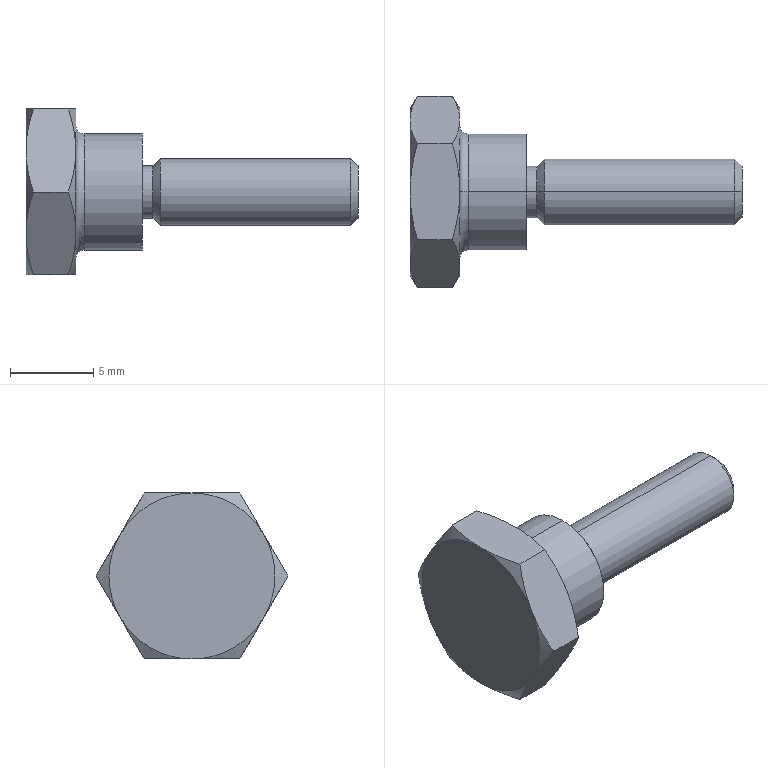Part | STEP file | 11-FJTM4_0_7_413part111 | 1 solid | 34 faces | box 20 x 11.547 x 10 mm | volume 570.86 mm3 | cone 16 | plane 10 | cylinder 6 | torus 2 | commonest cylinder face diameters 3.141 x2 4 x2 7 x2
STEP:
#1=CARTESIAN_POINT('',(3.,0.,-4.));
#2=VERTEX_POINT('',#1);
#3=CARTESIAN_POINT('',(3.,0.,4.));
#4=VERTEX_POINT('',#3);
#5=CARTESIAN_POINT('',(3.,0.,0.));
#6=DIRECTION('',(-1.,0.,0.));
#7=DIRECTION('',(0.,0.,1.));
#8=AXIS2_PLACEMENT_3D('',#5,#6,#7);
#9=CIRCLE('',#8,4.);
#10=EDGE_CURVE('',#2,#4,#9,.T.);
#11=ORIENTED_EDGE('',*,*,#10,.F.);
#12=CARTESIAN_POINT('',(3.5,0.,-3.5));
#13=VERTEX_POINT('',#12);
#14=CARTESIAN_POINT('',(3.5,0.,-4.));
#15=DIRECTION('',(0.,1.,0.));
#16=DIRECTION('',(0.,0.,1.));
#17=AXIS2_PLACEMENT_3D('',#14,#15,#16);
#18=CIRCLE('',#17,0.5);
#19=EDGE_CURVE('',#2,#13,#18,.T.);
#20=ORIENTED_EDGE('',*,*,#19,.T.);
#21=CARTESIAN_POINT('',(3.5,0.,3.5));
#22=VERTEX_POINT('',#21);
#23=CARTESIAN_POINT('',(3.5,0.,0.));
#24=DIRECTION('',(-1.,0.,0.));
#25=DIRECTION('',(0.,0.,1.));
#26=AXIS2_PLACEMENT_3D('',#23,#24,#25);
#27=CIRCLE('',#26,3.5);
#28=EDGE_CURVE('',#13,#22,#27,.T.);
#29=ORIENTED_EDGE('',*,*,#28,.T.);
#30=CARTESIAN_POINT('',(3.5,0.,4.));
#31=DIRECTION('',(0.,-1.,0.));
#32=DIRECTION('',(0.,0.,-1.));
#33=AXIS2_PLACEMENT_3D('',#30,#31,#32);
#34=CIRCLE('',#33,0.5);
#35=EDGE_CURVE('',#4,#22,#34,.T.);
#36=ORIENTED_EDGE('',*,*,#35,.F.);
#37=EDGE_LOOP('',(#11,#20,#29,#36));
#38=FACE_OUTER_BOUND('',#37,.T.);
#39=CARTESIAN_POINT('',(3.5,0.,0.));
#40=DIRECTION('',(-1.,0.,0.));
#41=DIRECTION('',(0.,0.,1.));
#42=AXIS2_PLACEMENT_3D('',#39,#40,#41);
#43=TOROIDAL_SURFACE('',#42,4.,0.5);
#44=ADVANCED_FACE('',(#38),#43,.F.);
#45=CARTESIAN_POINT('',(7.,0.,3.5));
#46=VERTEX_POINT('',#45);
#47=CARTESIAN_POINT('',(7.,0.,-3.5));
#48=VERTEX_POINT('',#47);
#49=CARTESIAN_POINT('',(7.,0.,0.));
#50=DIRECTION('',(-1.,0.,0.));
#51=DIRECTION('',(0.,0.,1.));
#52=AXIS2_PLACEMENT_3D('',#49,#50,#51);
#53=CIRCLE('',#52,3.5);
#54=EDGE_CURVE('',#46,#48,#53,.T.);
#55=ORIENTED_EDGE('',*,*,#54,.T.);
#56=CARTESIAN_POINT('',(20.,0.,-3.5));
#57=DIRECTION('',(-1.,0.,0.));
#58=VECTOR('',#57,1000.);
#59=LINE('',#56,#58);
#60=EDGE_CURVE('',#48,#13,#59,.T.);
#61=ORIENTED_EDGE('',*,*,#60,.T.);
#62=CARTESIAN_POINT('',(3.5,0.,0.));
#63=DIRECTION('',(-1.,0.,0.));
#64=DIRECTION('',(0.,0.,1.));
#65=AXIS2_PLACEMENT_3D('',#62,#63,#64);
#66=CIRCLE('',#65,3.5);
#67=EDGE_CURVE('',#22,#13,#66,.T.);
#68=ORIENTED_EDGE('',*,*,#67,.F.);
#69=CARTESIAN_POINT('',(20.,0.,3.5));
#70=DIRECTION('',(-1.,0.,0.));
#71=VECTOR('',#70,1000.);
#72=LINE('',#69,#71);
#73=EDGE_CURVE('',#46,#22,#72,.T.);
#74=ORIENTED_EDGE('',*,*,#73,.F.);
#75=EDGE_LOOP('',(#55,#61,#68,#74));
#76=FACE_OUTER_BOUND('',#75,.T.);
#77=CARTESIAN_POINT('',(20.,0.,0.));
#78=DIRECTION('',(-1.,0.,0.));
#79=DIRECTION('',(0.,0.,1.));
#80=AXIS2_PLACEMENT_3D('',#77,#78,#79);
#81=CYLINDRICAL_SURFACE('',#80,3.5);
#82=ADVANCED_FACE('',(#76),#81,.T.);
#83=CARTESIAN_POINT('',(7.65,0.,1.571));
#84=VERTEX_POINT('',#83);
#85=CARTESIAN_POINT('',(7.65,0.,-1.571));
#86=VERTEX_POINT('',#85);
#87=CARTESIAN_POINT('',(7.65,0.,0.));
#88=DIRECTION('',(-1.,0.,0.));
#89=DIRECTION('',(0.,0.,1.));
#90=AXIS2_PLACEMENT_3D('',#87,#88,#89);
#91=CIRCLE('',#90,1.571);
#92=EDGE_CURVE('',#84,#86,#91,.T.);
#93=ORIENTED_EDGE('',*,*,#92,.T.);
#94=CARTESIAN_POINT('',(7.,0.,-1.571));
#95=VERTEX_POINT('',#94);
#96=CARTESIAN_POINT('',(20.,0.,-1.571));
#97=DIRECTION('',(-1.,0.,0.));
#98=VECTOR('',#97,1000.);
#99=LINE('',#96,#98);
#100=EDGE_CURVE('',#86,#95,#99,.T.);
#101=ORIENTED_EDGE('',*,*,#100,.T.);
#102=CARTESIAN_POINT('',(7.,0.,1.571));
#103=VERTEX_POINT('',#102);
#104=CARTESIAN_POINT('',(7.,0.,0.));
#105=DIRECTION('',(-1.,0.,0.));
#106=DIRECTION('',(0.,0.,1.));
#107=AXIS2_PLACEMENT_3D('',#104,#105,#106);
#108=CIRCLE('',#107,1.571);
#109=EDGE_CURVE('',#103,#95,#108,.T.);
#110=ORIENTED_EDGE('',*,*,#109,.F.);
#111=CARTESIAN_POINT('',(20.,0.,1.571));
#112=DIRECTION('',(-1.,0.,0.));
#113=VECTOR('',#112,1000.);
#114=LINE('',#111,#113);
#115=EDGE_CURVE('',#84,#103,#114,.T.);
#116=ORIENTED_EDGE('',*,*,#115,.F.);
#117=EDGE_LOOP('',(#93,#101,#110,#116));
#118=FACE_OUTER_BOUND('',#117,.T.);
#119=CARTESIAN_POINT('',(20.,0.,0.));
#120=DIRECTION('',(-1.,0.,0.));
#121=DIRECTION('',(0.,0.,1.));
#122=AXIS2_PLACEMENT_3D('',#119,#120,#121);
#123=CYLINDRICAL_SURFACE('',#122,1.571);
#124=ADVANCED_FACE('',(#118),#123,.T.);
#125=ORIENTED_EDGE('',*,*,#92,.F.);
#126=CARTESIAN_POINT('',(8.079,0.,2.));
#127=VERTEX_POINT('',#126);
#128=CARTESIAN_POINT('',(8.079,0.,2.));
#129=DIRECTION('',(0.7071,0.,0.7071));
#130=VECTOR('',#129,1000.);
#131=LINE('',#128,#130);
#132=EDGE_CURVE('',#84,#127,#131,.T.);
#133=ORIENTED_EDGE('',*,*,#132,.T.);
#134=CARTESIAN_POINT('',(8.079,0.,-2.));
#135=VERTEX_POINT('',#134);
#136=CARTESIAN_POINT('',(8.079,0.,0.));
#137=DIRECTION('',(-1.,0.,0.));
#138=DIRECTION('',(0.,0.,1.));
#139=AXIS2_PLACEMENT_3D('',#136,#137,#138);
#140=CIRCLE('',#139,2.);
#141=EDGE_CURVE('',#127,#135,#140,.T.);
#142=ORIENTED_EDGE('',*,*,#141,.T.);
#143=CARTESIAN_POINT('',(8.079,0.,-2.));
#144=DIRECTION('',(0.7071,0.,-0.7071));
#145=VECTOR('',#144,1000.);
#146=LINE('',#143,#145);
#147=EDGE_CURVE('',#86,#135,#146,.T.);
#148=ORIENTED_EDGE('',*,*,#147,.F.);
#149=EDGE_LOOP('',(#125,#133,#142,#148));
#150=FACE_OUTER_BOUND('',#149,.T.);
#151=CARTESIAN_POINT('',(8.079,0.,0.));
#152=DIRECTION('',(1.,0.,0.));
#153=DIRECTION('',(0.,0.,-1.));
#154=AXIS2_PLACEMENT_3D('',#151,#152,#153);
#155=CONICAL_SURFACE('',#154,2.,0.7854);
#156=ADVANCED_FACE('',(#150),#155,.T.);
#157=CARTESIAN_POINT('',(19.571,0.,2.));
#158=VERTEX_POINT('',#157);
#159=CARTESIAN_POINT('',(19.571,0.,-2.));
#160=VERTEX_POINT('',#159);
#161=CARTESIAN_POINT('',(19.571,0.,0.));
#162=DIRECTION('',(-1.,0.,0.));
#163=DIRECTION('',(0.,0.,1.));
#164=AXIS2_PLACEMENT_3D('',#161,#162,#163);
#165=CIRCLE('',#164,2.);
#166=EDGE_CURVE('',#158,#160,#165,.T.);
#167=ORIENTED_EDGE('',*,*,#166,.T.);
#168=CARTESIAN_POINT('',(20.,0.,-2.));
#169=DIRECTION('',(-1.,0.,0.));
#170=VECTOR('',#169,1000.);
#171=LINE('',#168,#170);
#172=EDGE_CURVE('',#160,#135,#171,.T.);
#173=ORIENTED_EDGE('',*,*,#172,.T.);
#174=ORIENTED_EDGE('',*,*,#141,.F.);
#175=CARTESIAN_POINT('',(20.,0.,2.));
#176=DIRECTION('',(-1.,0.,0.));
#177=VECTOR('',#176,1000.);
#178=LINE('',#175,#177);
#179=EDGE_CURVE('',#158,#127,#178,.T.);
#180=ORIENTED_EDGE('',*,*,#179,.F.);
#181=EDGE_LOOP('',(#167,#173,#174,#180));
#182=FACE_OUTER_BOUND('',#181,.T.);
#183=CARTESIAN_POINT('',(20.,0.,0.));
#184=DIRECTION('',(-1.,0.,0.));
#185=DIRECTION('',(0.,0.,1.));
#186=AXIS2_PLACEMENT_3D('',#183,#184,#185);
#187=CYLINDRICAL_SURFACE('',#186,2.);
#188=ADVANCED_FACE('',(#182),#187,.T.);
#189=CARTESIAN_POINT('',(20.,0.,1.571));
#190=VERTEX_POINT('',#189);
#191=CARTESIAN_POINT('',(20.,0.,-1.571));
#192=VERTEX_POINT('',#191);
#193=CARTESIAN_POINT('',(20.,0.,0.));
#194=DIRECTION('',(-1.,0.,0.));
#195=DIRECTION('',(0.,0.,1.));
#196=AXIS2_PLACEMENT_3D('',#193,#194,#195);
#197=CIRCLE('',#196,1.571);
#198=EDGE_CURVE('',#190,#192,#197,.T.);
#199=ORIENTED_EDGE('',*,*,#198,.T.);
#200=CARTESIAN_POINT('',(20.,0.,-1.571));
#201=DIRECTION('',(-0.7071,0.,-0.7071));
#202=VECTOR('',#201,1000.);
#203=LINE('',#200,#202);
#204=EDGE_CURVE('',#192,#160,#203,.T.);
#205=ORIENTED_EDGE('',*,*,#204,.T.);
#206=ORIENTED_EDGE('',*,*,#166,.F.);
#207=CARTESIAN_POINT('',(20.,0.,1.571));
#208=DIRECTION('',(-0.7071,0.,0.7071));
#209=VECTOR('',#208,1000.);
#210=LINE('',#207,#209);
#211=EDGE_CURVE('',#190,#158,#210,.T.);
#212=ORIENTED_EDGE('',*,*,#211,.F.);
#213=EDGE_LOOP('',(#199,#205,#206,#212));
#214=FACE_OUTER_BOUND('',#213,.T.);
#215=CARTESIAN_POINT('',(20.,0.,0.));
#216=DIRECTION('',(-1.,0.,0.));
#217=DIRECTION('',(0.,0.,1.));
#218=AXIS2_PLACEMENT_3D('',#215,#216,#217);
#219=CONICAL_SURFACE('',#218,1.571,0.7854);
#220=ADVANCED_FACE('',(#214),#219,.T.);
#221=CARTESIAN_POINT('',(3.,4.33,-2.5));
#222=VERTEX_POINT('',#221);
#223=CARTESIAN_POINT('',(2.553,5.774,0.));
#224=VERTEX_POINT('',#223);
#225=CARTESIAN_POINT('',(3.,4.33,-2.5));
#226=CARTESIAN_POINT('',(3.,4.453,-2.288));
#227=CARTESIAN_POINT('',(2.989,4.576,-2.075));
#228=CARTESIAN_POINT('',(2.949,4.819,-1.653));
#229=CARTESIAN_POINT('',(2.918,4.94,-1.444));
#230=CARTESIAN_POINT('',(2.802,5.3,-0.8193));
#231=CARTESIAN_POINT('',(2.689,5.538,-0.4079));
#232=CARTESIAN_POINT('',(2.553,5.774,0.));
#233=B_SPLINE_CURVE_WITH_KNOTS('',3,(#225,#226,#227,#228,#229,#230,#231,#232),.UNSPECIFIED.,.F.,.F.,(4,2,2,4),(0.002921,0.003649,0.004376,0.005831),.UNSPECIFIED.);
#234=EDGE_CURVE('',#222,#224,#233,.T.);
#235=ORIENTED_EDGE('',*,*,#234,.T.);
#236=CARTESIAN_POINT('',(3.,4.33,2.5));
#237=VERTEX_POINT('',#236);
#238=CARTESIAN_POINT('',(2.553,5.774,0.));
#239=CARTESIAN_POINT('',(2.826,5.301,0.8179));
#240=CARTESIAN_POINT('',(3.,4.822,1.648));
#241=CARTESIAN_POINT('',(3.,4.33,2.5));
#242=B_SPLINE_CURVE_WITH_KNOTS('',3,(#238,#239,#240,#241),.UNSPECIFIED.,.F.,.F.,(4,4),(0.000000238,0.002921),.UNSPECIFIED.);
#243=EDGE_CURVE('',#224,#237,#242,.T.);
#244=ORIENTED_EDGE('',*,*,#243,.T.);
#245=CARTESIAN_POINT('',(3.,0.,0.));
#246=DIRECTION('',(-1.,0.,0.));
#247=DIRECTION('',(0.,0.,1.));
#248=AXIS2_PLACEMENT_3D('',#245,#246,#247);
#249=CIRCLE('',#248,5.);
#250=EDGE_CURVE('',#237,#222,#249,.T.);
#251=ORIENTED_EDGE('',*,*,#250,.T.);
#252=EDGE_LOOP('',(#235,#244,#251));
#253=FACE_OUTER_BOUND('',#252,.T.);
#254=CARTESIAN_POINT('',(3.,0.,0.));
#255=DIRECTION('',(-1.,0.,0.));
#256=DIRECTION('',(0.,0.,1.));
#257=AXIS2_PLACEMENT_3D('',#254,#255,#256);
#258=CONICAL_SURFACE('',#257,5.,1.047);
#259=ADVANCED_FACE('',(#253),#258,.T.);
#260=CARTESIAN_POINT('',(3.,0.,5.));
#261=VERTEX_POINT('',#260);
#262=CARTESIAN_POINT('',(3.,0.,0.));
#263=DIRECTION('',(-1.,0.,0.));
#264=DIRECTION('',(0.,0.,1.));
#265=AXIS2_PLACEMENT_3D('',#262,#263,#264);
#266=CIRCLE('',#265,5.);
#267=EDGE_CURVE('',#261,#237,#266,.T.);
#268=ORIENTED_EDGE('',*,*,#267,.T.);
#269=CARTESIAN_POINT('',(2.553,2.887,5.));
#270=VERTEX_POINT('',#269);
#271=CARTESIAN_POINT('',(3.,4.33,2.5));
#272=CARTESIAN_POINT('',(3.,4.208,2.712));
#273=CARTESIAN_POINT('',(2.989,4.085,2.925));
#274=CARTESIAN_POINT('',(2.949,3.841,3.347));
#275=CARTESIAN_POINT('',(2.918,3.72,3.556));
#276=CARTESIAN_POINT('',(2.802,3.36,4.181));
#277=CARTESIAN_POINT('',(2.689,3.122,4.592));
#278=CARTESIAN_POINT('',(2.553,2.887,5.));
#279=B_SPLINE_CURVE_WITH_KNOTS('',3,(#271,#272,#273,#274,#275,#276,#277,#278),.UNSPECIFIED.,.F.,.F.,(4,2,2,4),(0.002921,0.003649,0.004376,0.005831),.UNSPECIFIED.);
#280=EDGE_CURVE('',#237,#270,#279,.T.);
#281=ORIENTED_EDGE('',*,*,#280,.T.);
#282=CARTESIAN_POINT('',(2.553,2.887,5.));
#283=CARTESIAN_POINT('',(2.688,2.42,5.));
#284=CARTESIAN_POINT('',(2.8,1.947,5.));
#285=CARTESIAN_POINT('',(2.957,0.9829,5.));
#286=CARTESIAN_POINT('',(3.,0.4882,5.));
#287=CARTESIAN_POINT('',(3.,0.,5.));
#288=B_SPLINE_CURVE_WITH_KNOTS('',3,(#282,#283,#284,#285,#286,#287),.UNSPECIFIED.,.F.,.F.,(4,2,4),(0.01267,0.01414,0.0156),.UNSPECIFIED.);
#289=EDGE_CURVE('',#270,#261,#288,.T.);
#290=ORIENTED_EDGE('',*,*,#289,.T.);
#291=EDGE_LOOP('',(#268,#281,#290));
#292=FACE_OUTER_BOUND('',#291,.T.);
#293=CARTESIAN_POINT('',(3.,0.,0.));
#294=DIRECTION('',(-1.,0.,0.));
#295=DIRECTION('',(0.,0.,1.));
#296=AXIS2_PLACEMENT_3D('',#293,#294,#295);
#297=CONICAL_SURFACE('',#296,5.,1.047);
#298=ADVANCED_FACE('',(#292),#297,.T.);
#299=CARTESIAN_POINT('',(3.,-4.33,2.5));
#300=VERTEX_POINT('',#299);
#301=CARTESIAN_POINT('',(3.,0.,0.));
#302=DIRECTION('',(-1.,0.,0.));
#303=DIRECTION('',(0.,0.,1.));
#304=AXIS2_PLACEMENT_3D('',#301,#302,#303);
#305=CIRCLE('',#304,5.);
#306=EDGE_CURVE('',#300,#261,#305,.T.);
#307=ORIENTED_EDGE('',*,*,#306,.T.);
#308=CARTESIAN_POINT('',(2.553,-2.887,5.));
#309=VERTEX_POINT('',#308);
#310=CARTESIAN_POINT('',(3.,0.,5.));
#311=CARTESIAN_POINT('',(3.,-0.4879,5.));
#312=CARTESIAN_POINT('',(2.958,-0.9725,5.));
#313=CARTESIAN_POINT('',(2.803,-1.936,5.));
#314=CARTESIAN_POINT('',(2.689,-2.417,5.));
#315=CARTESIAN_POINT('',(2.553,-2.887,5.));
#316=B_SPLINE_CURVE_WITH_KNOTS('',3,(#310,#311,#312,#313,#314,#315),.UNSPECIFIED.,.F.,.F.,(4,2,4),(0.0156,0.01706,0.01852),.UNSPECIFIED.);
#317=EDGE_CURVE('',#261,#309,#316,.T.);
#318=ORIENTED_EDGE('',*,*,#317,.T.);
#319=CARTESIAN_POINT('',(2.553,-2.887,5.));
#320=CARTESIAN_POINT('',(2.826,-3.359,4.182));
#321=CARTESIAN_POINT('',(3.,-3.838,3.352));
#322=CARTESIAN_POINT('',(3.,-4.33,2.5));
#323=B_SPLINE_CURVE_WITH_KNOTS('',3,(#319,#320,#321,#322),.UNSPECIFIED.,.F.,.F.,(4,4),(0.000000238,0.002921),.UNSPECIFIED.);
#324=EDGE_CURVE('',#309,#300,#323,.T.);
#325=ORIENTED_EDGE('',*,*,#324,.T.);
#326=EDGE_LOOP('',(#307,#318,#325));
#327=FACE_OUTER_BOUND('',#326,.T.);
#328=CARTESIAN_POINT('',(3.,0.,0.));
#329=DIRECTION('',(-1.,0.,0.));
#330=DIRECTION('',(0.,0.,1.));
#331=AXIS2_PLACEMENT_3D('',#328,#329,#330);
#332=CONICAL_SURFACE('',#331,5.,1.047);
#333=ADVANCED_FACE('',(#327),#332,.T.);
#334=CARTESIAN_POINT('',(3.,-4.33,-2.5));
#335=VERTEX_POINT('',#334);
#336=CARTESIAN_POINT('',(3.,0.,0.));
#337=DIRECTION('',(-1.,0.,0.));
#338=DIRECTION('',(0.,0.,1.));
#339=AXIS2_PLACEMENT_3D('',#336,#337,#338);
#340=CIRCLE('',#339,5.);
#341=EDGE_CURVE('',#335,#300,#340,.T.);
#342=ORIENTED_EDGE('',*,*,#341,.T.);
#343=CARTESIAN_POINT('',(2.553,-5.774,0.));
#344=VERTEX_POINT('',#343);
#345=CARTESIAN_POINT('',(3.,-4.33,2.5));
#346=CARTESIAN_POINT('',(3.,-4.453,2.288));
#347=CARTESIAN_POINT('',(2.989,-4.576,2.075));
#348=CARTESIAN_POINT('',(2.949,-4.819,1.653));
#349=CARTESIAN_POINT('',(2.918,-4.94,1.444));
#350=CARTESIAN_POINT('',(2.802,-5.3,0.8193));
#351=CARTESIAN_POINT('',(2.689,-5.538,0.4079));
#352=CARTESIAN_POINT('',(2.553,-5.774,0.));
#353=B_SPLINE_CURVE_WITH_KNOTS('',3,(#345,#346,#347,#348,#349,#350,#351,#352),.UNSPECIFIED.,.F.,.F.,(4,2,2,4),(0.002921,0.003649,0.004376,0.005831),.UNSPECIFIED.);
#354=EDGE_CURVE('',#300,#344,#353,.T.);
#355=ORIENTED_EDGE('',*,*,#354,.T.);
#356=CARTESIAN_POINT('',(2.553,-5.774,0.));
#357=CARTESIAN_POINT('',(2.826,-5.301,-0.8179));
#358=CARTESIAN_POINT('',(3.,-4.822,-1.648));
#359=CARTESIAN_POINT('',(3.,-4.33,-2.5));
#360=B_SPLINE_CURVE_WITH_KNOTS('',3,(#356,#357,#358,#359),.UNSPECIFIED.,.F.,.F.,(4,4),(0.000000238,0.002921),.UNSPECIFIED.);
#361=EDGE_CURVE('',#344,#335,#360,.T.);
#362=ORIENTED_EDGE('',*,*,#361,.T.);
#363=EDGE_LOOP('',(#342,#355,#362));
#364=FACE_OUTER_BOUND('',#363,.T.);
#365=CARTESIAN_POINT('',(3.,0.,0.));
#366=DIRECTION('',(-1.,0.,0.));
#367=DIRECTION('',(0.,0.,1.));
#368=AXIS2_PLACEMENT_3D('',#365,#366,#367);
#369=CONICAL_SURFACE('',#368,5.,1.047);
#370=ADVANCED_FACE('',(#364),#369,.T.);
#371=CARTESIAN_POINT('',(3.,0.,-5.));
#372=VERTEX_POINT('',#371);
#373=CARTESIAN_POINT('',(3.,0.,0.));
#374=DIRECTION('',(-1.,0.,0.));
#375=DIRECTION('',(0.,0.,1.));
#376=AXIS2_PLACEMENT_3D('',#373,#374,#375);
#377=CIRCLE('',#376,5.);
#378=EDGE_CURVE('',#372,#335,#377,.T.);
#379=ORIENTED_EDGE('',*,*,#378,.T.);
#380=CARTESIAN_POINT('',(2.553,-2.887,-5.));
#381=VERTEX_POINT('',#380);
#382=CARTESIAN_POINT('',(3.,-4.33,-2.5));
#383=CARTESIAN_POINT('',(3.,-4.208,-2.712));
#384=CARTESIAN_POINT('',(2.989,-4.085,-2.925));
#385=CARTESIAN_POINT('',(2.949,-3.841,-3.347));
#386=CARTESIAN_POINT('',(2.918,-3.72,-3.556));
#387=CARTESIAN_POINT('',(2.802,-3.36,-4.181));
#388=CARTESIAN_POINT('',(2.689,-3.122,-4.592));
#389=CARTESIAN_POINT('',(2.553,-2.887,-5.));
#390=B_SPLINE_CURVE_WITH_KNOTS('',3,(#382,#383,#384,#385,#386,#387,#388,#389),.UNSPECIFIED.,.F.,.F.,(4,2,2,4),(0.002921,0.003649,0.004376,0.005831),.UNSPECIFIED.);
#391=EDGE_CURVE('',#335,#381,#390,.T.);
#392=ORIENTED_EDGE('',*,*,#391,.T.);
#393=CARTESIAN_POINT('',(2.553,-2.887,-5.));
#394=CARTESIAN_POINT('',(2.689,-2.417,-5.));
#395=CARTESIAN_POINT('',(2.803,-1.936,-5.));
#396=CARTESIAN_POINT('',(2.958,-0.9725,-5.));
#397=CARTESIAN_POINT('',(3.,-0.4879,-5.));
#398=CARTESIAN_POINT('',(3.,0.,-5.));
#399=B_SPLINE_CURVE_WITH_KNOTS('',3,(#393,#394,#395,#396,#397,#398),.UNSPECIFIED.,.F.,.F.,(4,2,4),(0.00517,0.006631,0.008091),.UNSPECIFIED.);
#400=EDGE_CURVE('',#381,#372,#399,.T.);
#401=ORIENTED_EDGE('',*,*,#400,.T.);
#402=EDGE_LOOP('',(#379,#392,#401));
#403=FACE_OUTER_BOUND('',#402,.T.);
#404=CARTESIAN_POINT('',(3.,0.,0.));
#405=DIRECTION('',(-1.,0.,0.));
#406=DIRECTION('',(0.,0.,1.));
#407=AXIS2_PLACEMENT_3D('',#404,#405,#406);
#408=CONICAL_SURFACE('',#407,5.,1.047);
#409=ADVANCED_FACE('',(#403),#408,.T.);
#410=ORIENTED_EDGE('',*,*,#198,.F.);
#411=CARTESIAN_POINT('',(20.,0.,0.));
#412=DIRECTION('',(-1.,0.,0.));
#413=DIRECTION('',(0.,0.,1.));
#414=AXIS2_PLACEMENT_3D('',#411,#412,#413);
#415=CIRCLE('',#414,1.571);
#416=EDGE_CURVE('',#192,#190,#415,.T.);
#417=ORIENTED_EDGE('',*,*,#416,.F.);
#418=EDGE_LOOP('',(#410,#417));
#419=FACE_OUTER_BOUND('',#418,.T.);
#420=CARTESIAN_POINT('',(20.,1.571,0.));
#421=DIRECTION('',(-1.,0.,0.));
#422=DIRECTION('',(0.,0.,1.));
#423=AXIS2_PLACEMENT_3D('',#420,#421,#422);
#424=PLANE('',#423);
#425=ADVANCED_FACE('',(#419),#424,.F.);
#426=ORIENTED_EDGE('',*,*,#204,.F.);
#427=ORIENTED_EDGE('',*,*,#416,.T.);
#428=ORIENTED_EDGE('',*,*,#211,.T.);
#429=CARTESIAN_POINT('',(19.571,0.,0.));
#430=DIRECTION('',(-1.,0.,0.));
#431=DIRECTION('',(0.,0.,1.));
#432=AXIS2_PLACEMENT_3D('',#429,#430,#431);
#433=CIRCLE('',#432,2.);
#434=EDGE_CURVE('',#160,#158,#433,.T.);
#435=ORIENTED_EDGE('',*,*,#434,.F.);
#436=EDGE_LOOP('',(#426,#427,#428,#435));
#437=FACE_OUTER_BOUND('',#436,.T.);
#438=CARTESIAN_POINT('',(20.,0.,0.));
#439=DIRECTION('',(-1.,0.,0.));
#440=DIRECTION('',(0.,0.,1.));
#441=AXIS2_PLACEMENT_3D('',#438,#439,#440);
#442=CONICAL_SURFACE('',#441,1.571,0.7854);
#443=ADVANCED_FACE('',(#437),#442,.T.);
#444=ORIENTED_EDGE('',*,*,#172,.F.);
#445=ORIENTED_EDGE('',*,*,#434,.T.);
#446=ORIENTED_EDGE('',*,*,#179,.T.);
#447=CARTESIAN_POINT('',(8.079,0.,0.));
#448=DIRECTION('',(-1.,0.,0.));
#449=DIRECTION('',(0.,0.,1.));
#450=AXIS2_PLACEMENT_3D('',#447,#448,#449);
#451=CIRCLE('',#450,2.);
#452=EDGE_CURVE('',#135,#127,#451,.T.);
#453=ORIENTED_EDGE('',*,*,#452,.F.);
#454=EDGE_LOOP('',(#444,#445,#446,#453));
#455=FACE_OUTER_BOUND('',#454,.T.);
#456=CARTESIAN_POINT('',(20.,0.,0.));
#457=DIRECTION('',(-1.,0.,0.));
#458=DIRECTION('',(0.,0.,1.));
#459=AXIS2_PLACEMENT_3D('',#456,#457,#458);
#460=CYLINDRICAL_SURFACE('',#459,2.);
#461=ADVANCED_FACE('',(#455),#460,.T.);
#462=ORIENTED_EDGE('',*,*,#132,.F.);
#463=CARTESIAN_POINT('',(7.65,0.,0.));
#464=DIRECTION('',(-1.,0.,0.));
#465=DIRECTION('',(0.,0.,1.));
#466=AXIS2_PLACEMENT_3D('',#463,#464,#465);
#467=CIRCLE('',#466,1.571);
#468=EDGE_CURVE('',#86,#84,#467,.T.);
#469=ORIENTED_EDGE('',*,*,#468,.F.);
#470=ORIENTED_EDGE('',*,*,#147,.T.);
#471=ORIENTED_EDGE('',*,*,#452,.T.);
#472=EDGE_LOOP('',(#462,#469,#470,#471));
#473=FACE_OUTER_BOUND('',#472,.T.);
#474=CARTESIAN_POINT('',(8.079,0.,0.));
#475=DIRECTION('',(1.,0.,0.));
#476=DIRECTION('',(0.,0.,-1.));
#477=AXIS2_PLACEMENT_3D('',#474,#475,#476);
#478=CONICAL_SURFACE('',#477,2.,0.7854);
#479=ADVANCED_FACE('',(#473),#478,.T.);
#480=ORIENTED_EDGE('',*,*,#100,.F.);
#481=ORIENTED_EDGE('',*,*,#468,.T.);
#482=ORIENTED_EDGE('',*,*,#115,.T.);
#483=CARTESIAN_POINT('',(7.,0.,0.));
#484=DIRECTION('',(-1.,0.,0.));
#485=DIRECTION('',(0.,0.,1.));
#486=AXIS2_PLACEMENT_3D('',#483,#484,#485);
#487=CIRCLE('',#486,1.571);
#488=EDGE_CURVE('',#95,#103,#487,.T.);
#489=ORIENTED_EDGE('',*,*,#488,.F.);
#490=EDGE_LOOP('',(#480,#481,#482,#489));
#491=FACE_OUTER_BOUND('',#490,.T.);
#492=CARTESIAN_POINT('',(20.,0.,0.));
#493=DIRECTION('',(-1.,0.,0.));
#494=DIRECTION('',(0.,0.,1.));
#495=AXIS2_PLACEMENT_3D('',#492,#493,#494);
#496=CYLINDRICAL_SURFACE('',#495,1.571);
#497=ADVANCED_FACE('',(#491),#496,.T.);
#498=ORIENTED_EDGE('',*,*,#54,.F.);
#499=CARTESIAN_POINT('',(7.,0.,0.));
#500=DIRECTION('',(-1.,0.,0.));
#501=DIRECTION('',(0.,0.,1.));
#502=AXIS2_PLACEMENT_3D('',#499,#500,#501);
#503=CIRCLE('',#502,3.5);
#504=EDGE_CURVE('',#48,#46,#503,.T.);
#505=ORIENTED_EDGE('',*,*,#504,.F.);
#506=EDGE_LOOP('',(#498,#505));
#507=FACE_OUTER_BOUND('',#506,.T.);
#508=ORIENTED_EDGE('',*,*,#109,.T.);
#509=ORIENTED_EDGE('',*,*,#488,.T.);
#510=EDGE_LOOP('',(#508,#509));
#511=FACE_BOUND('',#510,.T.);
#512=CARTESIAN_POINT('',(7.,3.5,0.));
#513=DIRECTION('',(-1.,0.,0.));
#514=DIRECTION('',(0.,0.,1.));
#515=AXIS2_PLACEMENT_3D('',#512,#513,#514);
#516=PLANE('',#515);
#517=ADVANCED_FACE('',(#507,#511),#516,.F.);
#518=ORIENTED_EDGE('',*,*,#60,.F.);
#519=ORIENTED_EDGE('',*,*,#504,.T.);
#520=ORIENTED_EDGE('',*,*,#73,.T.);
#521=ORIENTED_EDGE('',*,*,#28,.F.);
#522=EDGE_LOOP('',(#518,#519,#520,#521));
#523=FACE_OUTER_BOUND('',#522,.T.);
#524=CARTESIAN_POINT('',(20.,0.,0.));
#525=DIRECTION('',(-1.,0.,0.));
#526=DIRECTION('',(0.,0.,1.));
#527=AXIS2_PLACEMENT_3D('',#524,#525,#526);
#528=CYLINDRICAL_SURFACE('',#527,3.5);
#529=ADVANCED_FACE('',(#523),#528,.T.);
#530=ORIENTED_EDGE('',*,*,#19,.F.);
#531=CARTESIAN_POINT('',(3.,0.,0.));
#532=DIRECTION('',(-1.,0.,0.));
#533=DIRECTION('',(0.,0.,1.));
#534=AXIS2_PLACEMENT_3D('',#531,#532,#533);
#535=CIRCLE('',#534,4.);
#536=EDGE_CURVE('',#4,#2,#535,.T.);
#537=ORIENTED_EDGE('',*,*,#536,.F.);
#538=ORIENTED_EDGE('',*,*,#35,.T.);
#539=ORIENTED_EDGE('',*,*,#67,.T.);
#540=EDGE_LOOP('',(#530,#537,#538,#539));
#541=FACE_OUTER_BOUND('',#540,.T.);
#542=CARTESIAN_POINT('',(3.5,0.,0.));
#543=DIRECTION('',(-1.,0.,0.));
#544=DIRECTION('',(0.,0.,1.));
#545=AXIS2_PLACEMENT_3D('',#542,#543,#544);
#546=TOROIDAL_SURFACE('',#545,4.,0.5);
#547=ADVANCED_FACE('',(#541),#546,.F.);
#548=ORIENTED_EDGE('',*,*,#267,.F.);
#549=ORIENTED_EDGE('',*,*,#306,.F.);
#550=ORIENTED_EDGE('',*,*,#341,.F.);
#551=ORIENTED_EDGE('',*,*,#378,.F.);
#552=CARTESIAN_POINT('',(3.,0.,0.));
#553=DIRECTION('',(-1.,0.,0.));
#554=DIRECTION('',(0.,0.,1.));
#555=AXIS2_PLACEMENT_3D('',#552,#553,#554);
#556=CIRCLE('',#555,5.);
#557=EDGE_CURVE('',#222,#372,#556,.T.);
#558=ORIENTED_EDGE('',*,*,#557,.F.);
#559=ORIENTED_EDGE('',*,*,#250,.F.);
#560=EDGE_LOOP('',(#548,#549,#550,#551,#558,#559));
#561=FACE_OUTER_BOUND('',#560,.T.);
#562=ORIENTED_EDGE('',*,*,#536,.T.);
#563=ORIENTED_EDGE('',*,*,#10,.T.);
#564=EDGE_LOOP('',(#562,#563));
#565=FACE_BOUND('',#564,.T.);
#566=CARTESIAN_POINT('',(3.,5.,0.));
#567=DIRECTION('',(-1.,0.,0.));
#568=DIRECTION('',(0.,0.,1.));
#569=AXIS2_PLACEMENT_3D('',#566,#567,#568);
#570=PLANE('',#569);
#571=ADVANCED_FACE('',(#561,#565),#570,.F.);
#572=ORIENTED_EDGE('',*,*,#557,.T.);
#573=CARTESIAN_POINT('',(2.553,2.887,-5.));
#574=VERTEX_POINT('',#573);
#575=CARTESIAN_POINT('',(3.,0.,-5.));
#576=CARTESIAN_POINT('',(3.,0.4882,-5.));
#577=CARTESIAN_POINT('',(2.957,0.9829,-5.));
#578=CARTESIAN_POINT('',(2.8,1.947,-5.));
#579=CARTESIAN_POINT('',(2.688,2.42,-5.));
#580=CARTESIAN_POINT('',(2.553,2.887,-5.));
#581=B_SPLINE_CURVE_WITH_KNOTS('',3,(#575,#576,#577,#578,#579,#580),.UNSPECIFIED.,.F.,.F.,(4,2,4),(0.008091,0.009552,0.01101),.UNSPECIFIED.);
#582=EDGE_CURVE('',#372,#574,#581,.T.);
#583=ORIENTED_EDGE('',*,*,#582,.T.);
#584=CARTESIAN_POINT('',(2.553,2.887,-5.));
#585=CARTESIAN_POINT('',(2.826,3.359,-4.182));
#586=CARTESIAN_POINT('',(3.,3.838,-3.352));
#587=CARTESIAN_POINT('',(3.,4.33,-2.5));
#588=B_SPLINE_CURVE_WITH_KNOTS('',3,(#584,#585,#586,#587),.UNSPECIFIED.,.F.,.F.,(4,4),(0.000000238,0.002921),.UNSPECIFIED.);
#589=EDGE_CURVE('',#574,#222,#588,.T.);
#590=ORIENTED_EDGE('',*,*,#589,.T.);
#591=EDGE_LOOP('',(#572,#583,#590));
#592=FACE_OUTER_BOUND('',#591,.T.);
#593=CARTESIAN_POINT('',(3.,0.,0.));
#594=DIRECTION('',(-1.,0.,0.));
#595=DIRECTION('',(0.,0.,1.));
#596=AXIS2_PLACEMENT_3D('',#593,#594,#595);
#597=CONICAL_SURFACE('',#596,5.,1.047);
#598=ADVANCED_FACE('',(#592),#597,.T.);
#599=CARTESIAN_POINT('',(0.4466,5.774,0.));
#600=VERTEX_POINT('',#599);
#601=CARTESIAN_POINT('',(3.3,5.774,0.));
#602=DIRECTION('',(-1.,0.,0.));
#603=VECTOR('',#602,1000.);
#604=LINE('',#601,#603);
#605=EDGE_CURVE('',#224,#600,#604,.T.);
#606=ORIENTED_EDGE('',*,*,#605,.T.);
#607=CARTESIAN_POINT('',(0.,4.33,2.5));
#608=VERTEX_POINT('',#607);
#609=CARTESIAN_POINT('',(0.,4.33,2.5));
#610=CARTESIAN_POINT('',(0.,4.453,2.288));
#611=CARTESIAN_POINT('',(0.01056,4.576,2.075));
#612=CARTESIAN_POINT('',(0.0514,4.819,1.653));
#613=CARTESIAN_POINT('',(0.08166,4.94,1.444));
#614=CARTESIAN_POINT('',(0.1983,5.3,0.8193));
#615=CARTESIAN_POINT('',(0.3106,5.538,0.4079));
#616=CARTESIAN_POINT('',(0.4466,5.774,0.));
#617=B_SPLINE_CURVE_WITH_KNOTS('',3,(#609,#610,#611,#612,#613,#614,#615,#616),.UNSPECIFIED.,.F.,.F.,(4,2,2,4),(0.002921,0.003649,0.004376,0.005831),.UNSPECIFIED.);
#618=EDGE_CURVE('',#608,#600,#617,.T.);
#619=ORIENTED_EDGE('',*,*,#618,.F.);
#620=CARTESIAN_POINT('',(0.4466,2.887,5.));
#621=VERTEX_POINT('',#620);
#622=CARTESIAN_POINT('',(0.4466,2.887,5.));
#623=CARTESIAN_POINT('',(0.1739,3.359,4.182));
#624=CARTESIAN_POINT('',(0.,3.838,3.352));
#625=CARTESIAN_POINT('',(0.,4.33,2.5));
#626=B_SPLINE_CURVE_WITH_KNOTS('',3,(#622,#623,#624,#625),.UNSPECIFIED.,.F.,.F.,(4,4),(0.000000238,0.002921),.UNSPECIFIED.);
#627=EDGE_CURVE('',#621,#608,#626,.T.);
#628=ORIENTED_EDGE('',*,*,#627,.F.);
#629=CARTESIAN_POINT('',(3.3,2.887,5.));
#630=DIRECTION('',(-1.,0.,0.));
#631=VECTOR('',#630,1000.);
#632=LINE('',#629,#631);
#633=EDGE_CURVE('',#270,#621,#632,.T.);
#634=ORIENTED_EDGE('',*,*,#633,.F.);
#635=ORIENTED_EDGE('',*,*,#280,.F.);
#636=ORIENTED_EDGE('',*,*,#243,.F.);
#637=EDGE_LOOP('',(#606,#619,#628,#634,#635,#636));
#638=FACE_OUTER_BOUND('',#637,.T.);
#639=CARTESIAN_POINT('',(3.3,5.774,0.));
#640=DIRECTION('',(0.,-0.866,-0.5));
#641=DIRECTION('',(0.,0.5,-0.866));
#642=AXIS2_PLACEMENT_3D('',#639,#640,#641);
#643=PLANE('',#642);
#644=ADVANCED_FACE('',(#638),#643,.F.);
#645=ORIENTED_EDGE('',*,*,#633,.T.);
#646=CARTESIAN_POINT('',(0.,0.,5.));
#647=VERTEX_POINT('',#646);
#648=CARTESIAN_POINT('',(0.,0.,5.));
#649=CARTESIAN_POINT('',(0.,0.4882,5.));
#650=CARTESIAN_POINT('',(0.0431,0.9829,5.));
#651=CARTESIAN_POINT('',(0.1996,1.947,5.));
#652=CARTESIAN_POINT('',(0.3118,2.42,5.));
#653=CARTESIAN_POINT('',(0.4466,2.887,5.));
#654=B_SPLINE_CURVE_WITH_KNOTS('',3,(#648,#649,#650,#651,#652,#653),.UNSPECIFIED.,.F.,.F.,(4,2,4),(0.008091,0.009552,0.01101),.UNSPECIFIED.);
#655=EDGE_CURVE('',#647,#621,#654,.T.);
#656=ORIENTED_EDGE('',*,*,#655,.F.);
#657=CARTESIAN_POINT('',(0.4466,-2.887,5.));
#658=VERTEX_POINT('',#657);
#659=CARTESIAN_POINT('',(0.4466,-2.887,5.));
#660=CARTESIAN_POINT('',(0.311,-2.417,5.));
#661=CARTESIAN_POINT('',(0.1974,-1.936,5.));
#662=CARTESIAN_POINT('',(0.04194,-0.9725,5.));
#663=CARTESIAN_POINT('',(0.,-0.4879,5.));
#664=CARTESIAN_POINT('',(0.,0.,5.));
#665=B_SPLINE_CURVE_WITH_KNOTS('',3,(#659,#660,#661,#662,#663,#664),.UNSPECIFIED.,.F.,.F.,(4,2,4),(0.00517,0.006631,0.008091),.UNSPECIFIED.);
#666=EDGE_CURVE('',#658,#647,#665,.T.);
#667=ORIENTED_EDGE('',*,*,#666,.F.);
#668=CARTESIAN_POINT('',(3.3,-2.887,5.));
#669=DIRECTION('',(-1.,0.,0.));
#670=VECTOR('',#669,1000.);
#671=LINE('',#668,#670);
#672=EDGE_CURVE('',#309,#658,#671,.T.);
#673=ORIENTED_EDGE('',*,*,#672,.F.);
#674=ORIENTED_EDGE('',*,*,#317,.F.);
#675=ORIENTED_EDGE('',*,*,#289,.F.);
#676=EDGE_LOOP('',(#645,#656,#667,#673,#674,#675));
#677=FACE_OUTER_BOUND('',#676,.T.);
#678=CARTESIAN_POINT('',(3.3,2.887,5.));
#679=DIRECTION('',(0.,0.,-1.));
#680=DIRECTION('',(-1.,0.,0.));
#681=AXIS2_PLACEMENT_3D('',#678,#679,#680);
#682=PLANE('',#681);
#683=ADVANCED_FACE('',(#677),#682,.F.);
#684=ORIENTED_EDGE('',*,*,#672,.T.);
#685=CARTESIAN_POINT('',(0.,-4.33,2.5));
#686=VERTEX_POINT('',#685);
#687=CARTESIAN_POINT('',(0.,-4.33,2.5));
#688=CARTESIAN_POINT('',(0.,-4.208,2.712));
#689=CARTESIAN_POINT('',(0.01056,-4.085,2.925));
#690=CARTESIAN_POINT('',(0.0514,-3.841,3.347));
#691=CARTESIAN_POINT('',(0.08166,-3.72,3.556));
#692=CARTESIAN_POINT('',(0.1983,-3.36,4.181));
#693=CARTESIAN_POINT('',(0.3106,-3.122,4.592));
#694=CARTESIAN_POINT('',(0.4466,-2.887,5.));
#695=B_SPLINE_CURVE_WITH_KNOTS('',3,(#687,#688,#689,#690,#691,#692,#693,#694),.UNSPECIFIED.,.F.,.F.,(4,2,2,4),(0.002921,0.003649,0.004376,0.005831),.UNSPECIFIED.);
#696=EDGE_CURVE('',#686,#658,#695,.T.);
#697=ORIENTED_EDGE('',*,*,#696,.F.);
#698=CARTESIAN_POINT('',(0.4466,-5.774,0.));
#699=VERTEX_POINT('',#698);
#700=CARTESIAN_POINT('',(0.4466,-5.774,0.));
#701=CARTESIAN_POINT('',(0.1739,-5.301,0.8179));
#702=CARTESIAN_POINT('',(0.,-4.822,1.648));
#703=CARTESIAN_POINT('',(0.,-4.33,2.5));
#704=B_SPLINE_CURVE_WITH_KNOTS('',3,(#700,#701,#702,#703),.UNSPECIFIED.,.F.,.F.,(4,4),(0.000000238,0.002921),.UNSPECIFIED.);
#705=EDGE_CURVE('',#699,#686,#704,.T.);
#706=ORIENTED_EDGE('',*,*,#705,.F.);
#707=CARTESIAN_POINT('',(3.3,-5.774,0.));
#708=DIRECTION('',(-1.,0.,0.));
#709=VECTOR('',#708,1000.);
#710=LINE('',#707,#709);
#711=EDGE_CURVE('',#344,#699,#710,.T.);
#712=ORIENTED_EDGE('',*,*,#711,.F.);
#713=ORIENTED_EDGE('',*,*,#354,.F.);
#714=ORIENTED_EDGE('',*,*,#324,.F.);
#715=EDGE_LOOP('',(#684,#697,#706,#712,#713,#714));
#716=FACE_OUTER_BOUND('',#715,.T.);
#717=CARTESIAN_POINT('',(3.3,-2.887,5.));
#718=DIRECTION('',(0.,0.866,-0.5));
#719=DIRECTION('',(0.,0.5,0.866));
#720=AXIS2_PLACEMENT_3D('',#717,#718,#719);
#721=PLANE('',#720);
#722=ADVANCED_FACE('',(#716),#721,.F.);
#723=ORIENTED_EDGE('',*,*,#711,.T.);
#724=CARTESIAN_POINT('',(0.,-4.33,-2.5));
#725=VERTEX_POINT('',#724);
#726=CARTESIAN_POINT('',(0.,-4.33,-2.5));
#727=CARTESIAN_POINT('',(0.,-4.453,-2.288));
#728=CARTESIAN_POINT('',(0.01056,-4.576,-2.075));
#729=CARTESIAN_POINT('',(0.0514,-4.819,-1.653));
#730=CARTESIAN_POINT('',(0.08166,-4.94,-1.444));
#731=CARTESIAN_POINT('',(0.1983,-5.3,-0.8193));
#732=CARTESIAN_POINT('',(0.3106,-5.538,-0.4079));
#733=CARTESIAN_POINT('',(0.4466,-5.774,0.));
#734=B_SPLINE_CURVE_WITH_KNOTS('',3,(#726,#727,#728,#729,#730,#731,#732,#733),.UNSPECIFIED.,.F.,.F.,(4,2,2,4),(0.002921,0.003649,0.004376,0.005831),.UNSPECIFIED.);
#735=EDGE_CURVE('',#725,#699,#734,.T.);
#736=ORIENTED_EDGE('',*,*,#735,.F.);
#737=CARTESIAN_POINT('',(0.4466,-2.887,-5.));
#738=VERTEX_POINT('',#737);
#739=CARTESIAN_POINT('',(0.4466,-2.887,-5.));
#740=CARTESIAN_POINT('',(0.1739,-3.359,-4.182));
#741=CARTESIAN_POINT('',(0.,-3.838,-3.352));
#742=CARTESIAN_POINT('',(0.,-4.33,-2.5));
#743=B_SPLINE_CURVE_WITH_KNOTS('',3,(#739,#740,#741,#742),.UNSPECIFIED.,.F.,.F.,(4,4),(0.000000238,0.002921),.UNSPECIFIED.);
#744=EDGE_CURVE('',#738,#725,#743,.T.);
#745=ORIENTED_EDGE('',*,*,#744,.F.);
#746=CARTESIAN_POINT('',(3.3,-2.887,-5.));
#747=DIRECTION('',(-1.,0.,0.));
#748=VECTOR('',#747,1000.);
#749=LINE('',#746,#748);
#750=EDGE_CURVE('',#381,#738,#749,.T.);
#751=ORIENTED_EDGE('',*,*,#750,.F.);
#752=ORIENTED_EDGE('',*,*,#391,.F.);
#753=ORIENTED_EDGE('',*,*,#361,.F.);
#754=EDGE_LOOP('',(#723,#736,#745,#751,#752,#753));
#755=FACE_OUTER_BOUND('',#754,.T.);
#756=CARTESIAN_POINT('',(3.3,-5.774,0.));
#757=DIRECTION('',(0.,0.866,0.5));
#758=DIRECTION('',(0.,-0.5,0.866));
#759=AXIS2_PLACEMENT_3D('',#756,#757,#758);
#760=PLANE('',#759);
#761=ADVANCED_FACE('',(#755),#760,.F.);
#762=ORIENTED_EDGE('',*,*,#750,.T.);
#763=CARTESIAN_POINT('',(0.,0.,-5.));
#764=VERTEX_POINT('',#763);
#765=CARTESIAN_POINT('',(0.,0.,-5.));
#766=CARTESIAN_POINT('',(0.,-0.4879,-5.));
#767=CARTESIAN_POINT('',(0.04194,-0.9725,-5.));
#768=CARTESIAN_POINT('',(0.1974,-1.936,-5.));
#769=CARTESIAN_POINT('',(0.311,-2.417,-5.));
#770=CARTESIAN_POINT('',(0.4466,-2.887,-5.));
#771=B_SPLINE_CURVE_WITH_KNOTS('',3,(#765,#766,#767,#768,#769,#770),.UNSPECIFIED.,.F.,.F.,(4,2,4),(0.0156,0.01706,0.01852),.UNSPECIFIED.);
#772=EDGE_CURVE('',#764,#738,#771,.T.);
#773=ORIENTED_EDGE('',*,*,#772,.F.);
#774=CARTESIAN_POINT('',(0.4466,2.887,-5.));
#775=VERTEX_POINT('',#774);
#776=CARTESIAN_POINT('',(0.4466,2.887,-5.));
#777=CARTESIAN_POINT('',(0.3118,2.42,-5.));
#778=CARTESIAN_POINT('',(0.1996,1.947,-5.));
#779=CARTESIAN_POINT('',(0.0431,0.9829,-5.));
#780=CARTESIAN_POINT('',(0.,0.4882,-5.));
#781=CARTESIAN_POINT('',(0.,0.,-5.));
#782=B_SPLINE_CURVE_WITH_KNOTS('',3,(#776,#777,#778,#779,#780,#781),.UNSPECIFIED.,.F.,.F.,(4,2,4),(0.01267,0.01414,0.0156),.UNSPECIFIED.);
#783=EDGE_CURVE('',#775,#764,#782,.T.);
#784=ORIENTED_EDGE('',*,*,#783,.F.);
#785=CARTESIAN_POINT('',(3.3,2.887,-5.));
#786=DIRECTION('',(-1.,0.,0.));
#787=VECTOR('',#786,1000.);
#788=LINE('',#785,#787);
#789=EDGE_CURVE('',#574,#775,#788,.T.);
#790=ORIENTED_EDGE('',*,*,#789,.F.);
#791=ORIENTED_EDGE('',*,*,#582,.F.);
#792=ORIENTED_EDGE('',*,*,#400,.F.);
#793=EDGE_LOOP('',(#762,#773,#784,#790,#791,#792));
#794=FACE_OUTER_BOUND('',#793,.T.);
#795=CARTESIAN_POINT('',(3.3,-2.887,-5.));
#796=DIRECTION('',(0.,0.,1.));
#797=DIRECTION('',(1.,0.,0.));
#798=AXIS2_PLACEMENT_3D('',#795,#796,#797);
#799=PLANE('',#798);
#800=ADVANCED_FACE('',(#794),#799,.F.);
#801=ORIENTED_EDGE('',*,*,#789,.T.);
#802=CARTESIAN_POINT('',(0.,4.33,-2.5));
#803=VERTEX_POINT('',#802);
#804=CARTESIAN_POINT('',(0.,4.33,-2.5));
#805=CARTESIAN_POINT('',(0.,4.208,-2.712));
#806=CARTESIAN_POINT('',(0.01056,4.085,-2.925));
#807=CARTESIAN_POINT('',(0.0514,3.841,-3.347));
#808=CARTESIAN_POINT('',(0.08166,3.72,-3.556));
#809=CARTESIAN_POINT('',(0.1983,3.36,-4.181));
#810=CARTESIAN_POINT('',(0.3106,3.122,-4.592));
#811=CARTESIAN_POINT('',(0.4466,2.887,-5.));
#812=B_SPLINE_CURVE_WITH_KNOTS('',3,(#804,#805,#806,#807,#808,#809,#810,#811),.UNSPECIFIED.,.F.,.F.,(4,2,2,4),(0.002921,0.003649,0.004376,0.005831),.UNSPECIFIED.);
#813=EDGE_CURVE('',#803,#775,#812,.T.);
#814=ORIENTED_EDGE('',*,*,#813,.F.);
#815=CARTESIAN_POINT('',(0.4466,5.774,0.));
#816=CARTESIAN_POINT('',(0.1739,5.301,-0.8179));
#817=CARTESIAN_POINT('',(0.,4.822,-1.648));
#818=CARTESIAN_POINT('',(0.,4.33,-2.5));
#819=B_SPLINE_CURVE_WITH_KNOTS('',3,(#815,#816,#817,#818),.UNSPECIFIED.,.F.,.F.,(4,4),(0.000000238,0.002921),.UNSPECIFIED.);
#820=EDGE_CURVE('',#600,#803,#819,.T.);
#821=ORIENTED_EDGE('',*,*,#820,.F.);
#822=ORIENTED_EDGE('',*,*,#605,.F.);
#823=ORIENTED_EDGE('',*,*,#234,.F.);
#824=ORIENTED_EDGE('',*,*,#589,.F.);
#825=EDGE_LOOP('',(#801,#814,#821,#822,#823,#824));
#826=FACE_OUTER_BOUND('',#825,.T.);
#827=CARTESIAN_POINT('',(3.3,2.887,-5.));
#828=DIRECTION('',(0.,-0.866,0.5));
#829=DIRECTION('',(0.,-0.5,-0.866));
#830=AXIS2_PLACEMENT_3D('',#827,#828,#829);
#831=PLANE('',#830);
#832=ADVANCED_FACE('',(#826),#831,.F.);
#833=CARTESIAN_POINT('',(0.,0.,0.));
#834=DIRECTION('',(-1.,0.,0.));
#835=DIRECTION('',(0.,0.,1.));
#836=AXIS2_PLACEMENT_3D('',#833,#834,#835);
#837=CIRCLE('',#836,5.);
#838=EDGE_CURVE('',#686,#647,#837,.T.);
#839=ORIENTED_EDGE('',*,*,#838,.F.);
#840=ORIENTED_EDGE('',*,*,#696,.T.);
#841=ORIENTED_EDGE('',*,*,#666,.T.);
#842=EDGE_LOOP('',(#839,#840,#841));
#843=FACE_OUTER_BOUND('',#842,.T.);
#844=CARTESIAN_POINT('',(0.5774,0.,0.));
#845=DIRECTION('',(1.,0.,0.));
#846=DIRECTION('',(0.,0.,-1.));
#847=AXIS2_PLACEMENT_3D('',#844,#845,#846);
#848=CONICAL_SURFACE('',#847,6.,1.047);
#849=ADVANCED_FACE('',(#843),#848,.T.);
#850=ORIENTED_EDGE('',*,*,#735,.T.);
#851=ORIENTED_EDGE('',*,*,#705,.T.);
#852=CARTESIAN_POINT('',(0.,0.,0.));
#853=DIRECTION('',(-1.,0.,0.));
#854=DIRECTION('',(0.,0.,1.));
#855=AXIS2_PLACEMENT_3D('',#852,#853,#854);
#856=CIRCLE('',#855,5.);
#857=EDGE_CURVE('',#725,#686,#856,.T.);
#858=ORIENTED_EDGE('',*,*,#857,.F.);
#859=EDGE_LOOP('',(#850,#851,#858));
#860=FACE_OUTER_BOUND('',#859,.T.);
#861=CARTESIAN_POINT('',(0.5774,0.,0.));
#862=DIRECTION('',(1.,0.,0.));
#863=DIRECTION('',(0.,0.,-1.));
#864=AXIS2_PLACEMENT_3D('',#861,#862,#863);
#865=CONICAL_SURFACE('',#864,6.,1.047);
#866=ADVANCED_FACE('',(#860),#865,.T.);
#867=ORIENTED_EDGE('',*,*,#772,.T.);
#868=ORIENTED_EDGE('',*,*,#744,.T.);
#869=CARTESIAN_POINT('',(0.,0.,0.));
#870=DIRECTION('',(-1.,0.,0.));
#871=DIRECTION('',(0.,0.,1.));
#872=AXIS2_PLACEMENT_3D('',#869,#870,#871);
#873=CIRCLE('',#872,5.);
#874=EDGE_CURVE('',#764,#725,#873,.T.);
#875=ORIENTED_EDGE('',*,*,#874,.F.);
#876=EDGE_LOOP('',(#867,#868,#875));
#877=FACE_OUTER_BOUND('',#876,.T.);
#878=CARTESIAN_POINT('',(0.5774,0.,0.));
#879=DIRECTION('',(1.,0.,0.));
#880=DIRECTION('',(0.,0.,-1.));
#881=AXIS2_PLACEMENT_3D('',#878,#879,#880);
#882=CONICAL_SURFACE('',#881,6.,1.047);
#883=ADVANCED_FACE('',(#877),#882,.T.);
#884=CARTESIAN_POINT('',(0.,0.,0.));
#885=DIRECTION('',(-1.,0.,0.));
#886=DIRECTION('',(0.,0.,1.));
#887=AXIS2_PLACEMENT_3D('',#884,#885,#886);
#888=CIRCLE('',#887,5.);
#889=EDGE_CURVE('',#608,#803,#888,.T.);
#890=ORIENTED_EDGE('',*,*,#889,.F.);
#891=ORIENTED_EDGE('',*,*,#618,.T.);
#892=ORIENTED_EDGE('',*,*,#820,.T.);
#893=EDGE_LOOP('',(#890,#891,#892));
#894=FACE_OUTER_BOUND('',#893,.T.);
#895=CARTESIAN_POINT('',(0.5774,0.,0.));
#896=DIRECTION('',(1.,0.,0.));
#897=DIRECTION('',(0.,0.,-1.));
#898=AXIS2_PLACEMENT_3D('',#895,#896,#897);
#899=CONICAL_SURFACE('',#898,6.,1.047);
#900=ADVANCED_FACE('',(#894),#899,.T.);
#901=CARTESIAN_POINT('',(0.,0.,0.));
#902=DIRECTION('',(-1.,0.,0.));
#903=DIRECTION('',(0.,0.,1.));
#904=AXIS2_PLACEMENT_3D('',#901,#902,#903);
#905=CIRCLE('',#904,5.);
#906=EDGE_CURVE('',#647,#608,#905,.T.);
#907=ORIENTED_EDGE('',*,*,#906,.F.);
#908=ORIENTED_EDGE('',*,*,#655,.T.);
#909=ORIENTED_EDGE('',*,*,#627,.T.);
#910=EDGE_LOOP('',(#907,#908,#909));
#911=FACE_OUTER_BOUND('',#910,.T.);
#912=CARTESIAN_POINT('',(0.5774,0.,0.));
#913=DIRECTION('',(1.,0.,0.));
#914=DIRECTION('',(0.,0.,-1.));
#915=AXIS2_PLACEMENT_3D('',#912,#913,#914);
#916=CONICAL_SURFACE('',#915,6.,1.047);
#917=ADVANCED_FACE('',(#911),#916,.T.);
#918=ORIENTED_EDGE('',*,*,#906,.T.);
#919=ORIENTED_EDGE('',*,*,#889,.T.);
#920=CARTESIAN_POINT('',(0.,0.,0.));
#921=DIRECTION('',(-1.,0.,0.));
#922=DIRECTION('',(0.,0.,1.));
#923=AXIS2_PLACEMENT_3D('',#920,#921,#922);
#924=CIRCLE('',#923,5.);
#925=EDGE_CURVE('',#803,#764,#924,.T.);
#926=ORIENTED_EDGE('',*,*,#925,.T.);
#927=ORIENTED_EDGE('',*,*,#874,.T.);
#928=ORIENTED_EDGE('',*,*,#857,.T.);
#929=ORIENTED_EDGE('',*,*,#838,.T.);
#930=EDGE_LOOP('',(#918,#919,#926,#927,#928,#929));
#931=FACE_OUTER_BOUND('',#930,.T.);
#932=CARTESIAN_POINT('',(0.,0.,0.));
#933=DIRECTION('',(1.,0.,0.));
#934=DIRECTION('',(0.,0.,-1.));
#935=AXIS2_PLACEMENT_3D('',#932,#933,#934);
#936=PLANE('',#935);
#937=ADVANCED_FACE('',(#931),#936,.F.);
#938=ORIENTED_EDGE('',*,*,#813,.T.);
#939=ORIENTED_EDGE('',*,*,#783,.T.);
#940=ORIENTED_EDGE('',*,*,#925,.F.);
#941=EDGE_LOOP('',(#938,#939,#940));
#942=FACE_OUTER_BOUND('',#941,.T.);
#943=CARTESIAN_POINT('',(0.5774,0.,0.));
#944=DIRECTION('',(1.,0.,0.));
#945=DIRECTION('',(0.,0.,-1.));
#946=AXIS2_PLACEMENT_3D('',#943,#944,#945);
#947=CONICAL_SURFACE('',#946,6.,1.047);
#948=ADVANCED_FACE('',(#942),#947,.T.);
#949=CLOSED_SHELL('',(#44,#82,#124,#156,#188,#220,#259,#298,#333,#370,#409,#425,#443,#461,#479,#497,#517,#529,#547,#571,#598,#644,#683,#722,#761,#800,#832,#849,#866,#883,#900,#917,#937,#948));
#950=MANIFOLD_SOLID_BREP('',#949);
#951=CARTESIAN_POINT('',(0.,0.,0.));
#952=DIRECTION('',(0.,0.,1.));
#953=DIRECTION('',(1.,0.,0.));
#954=AXIS2_PLACEMENT_3D('',#951,#952,#953);
#955=(LENGTH_UNIT()NAMED_UNIT(*)SI_UNIT(.MILLI.,.METRE.));
#956=UNCERTAINTY_MEASURE_WITH_UNIT(LENGTH_MEASURE(0.00001),#955,'','');
#957=(NAMED_UNIT(*)PLANE_ANGLE_UNIT()SI_UNIT($,.RADIAN.));
#958=(NAMED_UNIT(*)SI_UNIT($,.STERADIAN.)SOLID_ANGLE_UNIT());
#959=(GEOMETRIC_REPRESENTATION_CONTEXT(3)GLOBAL_UNCERTAINTY_ASSIGNED_CONTEXT((#956))GLOBAL_UNIT_ASSIGNED_CONTEXT((#955,#957,#958))REPRESENTATION_CONTEXT('',''));
#960=ADVANCED_BREP_SHAPE_REPRESENTATION('',(#950,#954),#959);